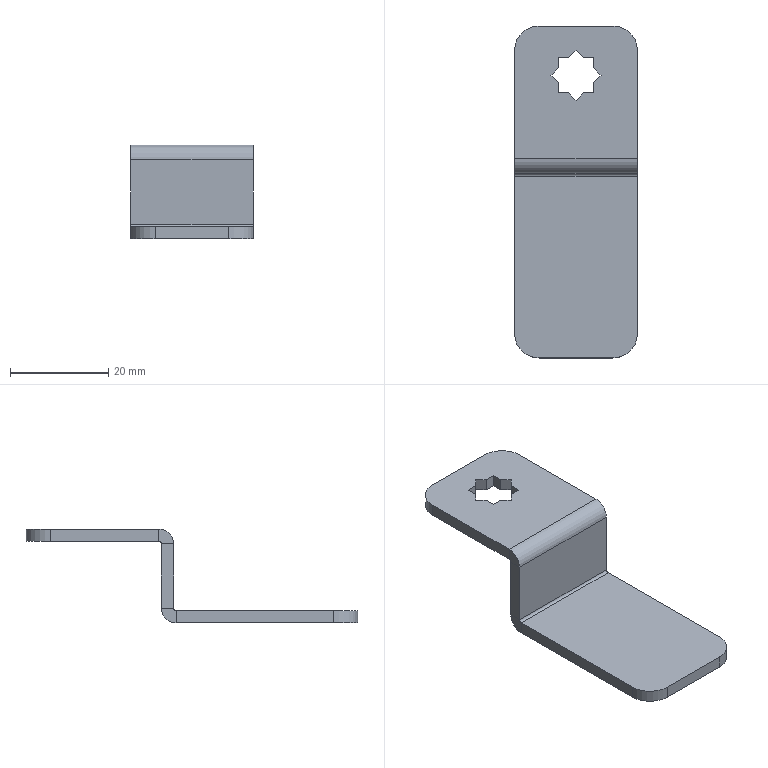Part | SolidWorks | features BaseBody 1 | 1 solid | 42 faces | box 25 x 67.5 x 19.1 mm | volume 4957 mm3 | plane 34 | cylinder 8 | commonest cylinder face diameters 10 x4 1 x2 6 x2
STEP:
#1=CARTESIAN_POINT('',(5.091,5.,0.));
#2=VERTEX_POINT('',#1);
#3=CARTESIAN_POINT('',(3.6,3.509,0.));
#4=VERTEX_POINT('',#3);
#5=CARTESIAN_POINT('',(5.091,5.,0.));
#6=DIRECTION('',(-0.7071,-0.7071,0.));
#7=VECTOR('',#6,1000.);
#8=LINE('',#5,#7);
#9=EDGE_CURVE('',#2,#4,#8,.T.);
#10=ORIENTED_EDGE('',*,*,#9,.F.);
#11=CARTESIAN_POINT('',(5.091,5.,-2.5));
#12=VERTEX_POINT('',#11);
#13=CARTESIAN_POINT('',(5.091,5.,0.));
#14=DIRECTION('',(0.,0.,-1.));
#15=VECTOR('',#14,1000.);
#16=LINE('',#13,#15);
#17=EDGE_CURVE('',#2,#12,#16,.T.);
#18=ORIENTED_EDGE('',*,*,#17,.T.);
#19=CARTESIAN_POINT('',(3.6,3.509,-2.5));
#20=VERTEX_POINT('',#19);
#21=CARTESIAN_POINT('',(5.091,5.,-2.5));
#22=DIRECTION('',(-0.7071,-0.7071,0.));
#23=VECTOR('',#22,1000.);
#24=LINE('',#21,#23);
#25=EDGE_CURVE('',#12,#20,#24,.T.);
#26=ORIENTED_EDGE('',*,*,#25,.T.);
#27=CARTESIAN_POINT('',(3.6,3.509,0.));
#28=DIRECTION('',(0.,0.,-1.));
#29=VECTOR('',#28,1000.);
#30=LINE('',#27,#29);
#31=EDGE_CURVE('',#4,#20,#30,.T.);
#32=ORIENTED_EDGE('',*,*,#31,.F.);
#33=EDGE_LOOP('',(#10,#18,#26,#32));
#34=FACE_OUTER_BOUND('',#33,.T.);
#35=CARTESIAN_POINT('',(5.091,5.,0.));
#36=DIRECTION('',(0.7071,-0.7071,0.));
#37=DIRECTION('',(0.,0.,-1.));
#38=AXIS2_PLACEMENT_3D('',#35,#36,#37);
#39=PLANE('',#38);
#40=ADVANCED_FACE('',(#34),#39,.F.);
#41=CARTESIAN_POINT('',(3.6,6.491,-2.5));
#42=VERTEX_POINT('',#41);
#43=CARTESIAN_POINT('',(0.,10.091,-2.5));
#44=DIRECTION('',(0.7071,-0.7071,0.));
#45=VECTOR('',#44,1000.);
#46=LINE('',#43,#45);
#47=EDGE_CURVE('',#42,#12,#46,.T.);
#48=ORIENTED_EDGE('',*,*,#47,.T.);
#49=ORIENTED_EDGE('',*,*,#17,.F.);
#50=CARTESIAN_POINT('',(3.6,6.491,0.));
#51=VERTEX_POINT('',#50);
#52=CARTESIAN_POINT('',(0.,10.091,0.));
#53=DIRECTION('',(0.7071,-0.7071,0.));
#54=VECTOR('',#53,1000.);
#55=LINE('',#52,#54);
#56=EDGE_CURVE('',#51,#2,#55,.T.);
#57=ORIENTED_EDGE('',*,*,#56,.F.);
#58=CARTESIAN_POINT('',(3.6,6.491,0.));
#59=DIRECTION('',(0.,0.,1.));
#60=VECTOR('',#59,1000.);
#61=LINE('',#58,#60);
#62=EDGE_CURVE('',#42,#51,#61,.T.);
#63=ORIENTED_EDGE('',*,*,#62,.F.);
#64=EDGE_LOOP('',(#48,#49,#57,#63));
#65=FACE_OUTER_BOUND('',#64,.T.);
#66=CARTESIAN_POINT('',(0.,10.091,0.));
#67=DIRECTION('',(0.7071,0.7071,0.));
#68=DIRECTION('',(0.,0.,-1.));
#69=AXIS2_PLACEMENT_3D('',#66,#67,#68);
#70=PLANE('',#69);
#71=ADVANCED_FACE('',(#65),#70,.F.);
#72=CARTESIAN_POINT('',(0.,10.091,0.));
#73=VERTEX_POINT('',#72);
#74=CARTESIAN_POINT('',(1.491,8.6,0.));
#75=VERTEX_POINT('',#74);
#76=CARTESIAN_POINT('',(0.,10.091,0.));
#77=DIRECTION('',(0.7071,-0.7071,0.));
#78=VECTOR('',#77,1000.);
#79=LINE('',#76,#78);
#80=EDGE_CURVE('',#73,#75,#79,.T.);
#81=ORIENTED_EDGE('',*,*,#80,.F.);
#82=CARTESIAN_POINT('',(0.,10.091,-2.5));
#83=VERTEX_POINT('',#82);
#84=CARTESIAN_POINT('',(0.,10.091,0.));
#85=DIRECTION('',(0.,0.,-1.));
#86=VECTOR('',#85,1000.);
#87=LINE('',#84,#86);
#88=EDGE_CURVE('',#73,#83,#87,.T.);
#89=ORIENTED_EDGE('',*,*,#88,.T.);
#90=CARTESIAN_POINT('',(1.491,8.6,-2.5));
#91=VERTEX_POINT('',#90);
#92=CARTESIAN_POINT('',(0.,10.091,-2.5));
#93=DIRECTION('',(0.7071,-0.7071,0.));
#94=VECTOR('',#93,1000.);
#95=LINE('',#92,#94);
#96=EDGE_CURVE('',#83,#91,#95,.T.);
#97=ORIENTED_EDGE('',*,*,#96,.T.);
#98=CARTESIAN_POINT('',(1.491,8.6,0.));
#99=DIRECTION('',(0.,0.,-1.));
#100=VECTOR('',#99,1000.);
#101=LINE('',#98,#100);
#102=EDGE_CURVE('',#75,#91,#101,.T.);
#103=ORIENTED_EDGE('',*,*,#102,.F.);
#104=EDGE_LOOP('',(#81,#89,#97,#103));
#105=FACE_OUTER_BOUND('',#104,.T.);
#106=CARTESIAN_POINT('',(0.,10.091,0.));
#107=DIRECTION('',(0.7071,0.7071,0.));
#108=DIRECTION('',(0.,0.,-1.));
#109=AXIS2_PLACEMENT_3D('',#106,#107,#108);
#110=PLANE('',#109);
#111=ADVANCED_FACE('',(#105),#110,.F.);
#112=CARTESIAN_POINT('',(-1.491,8.6,-2.5));
#113=VERTEX_POINT('',#112);
#114=CARTESIAN_POINT('',(0.,10.091,-2.5));
#115=DIRECTION('',(0.7071,0.7071,0.));
#116=VECTOR('',#115,1000.);
#117=LINE('',#114,#116);
#118=EDGE_CURVE('',#113,#83,#117,.T.);
#119=ORIENTED_EDGE('',*,*,#118,.T.);
#120=ORIENTED_EDGE('',*,*,#88,.F.);
#121=CARTESIAN_POINT('',(-1.491,8.6,0.));
#122=VERTEX_POINT('',#121);
#123=CARTESIAN_POINT('',(0.,10.091,0.));
#124=DIRECTION('',(0.7071,0.7071,0.));
#125=VECTOR('',#124,1000.);
#126=LINE('',#123,#125);
#127=EDGE_CURVE('',#122,#73,#126,.T.);
#128=ORIENTED_EDGE('',*,*,#127,.F.);
#129=CARTESIAN_POINT('',(-1.491,8.6,0.));
#130=DIRECTION('',(0.,0.,1.));
#131=VECTOR('',#130,1000.);
#132=LINE('',#129,#131);
#133=EDGE_CURVE('',#113,#122,#132,.T.);
#134=ORIENTED_EDGE('',*,*,#133,.F.);
#135=EDGE_LOOP('',(#119,#120,#128,#134));
#136=FACE_OUTER_BOUND('',#135,.T.);
#137=CARTESIAN_POINT('',(0.,10.091,0.));
#138=DIRECTION('',(-0.7071,0.7071,0.));
#139=DIRECTION('',(0.,0.,1.));
#140=AXIS2_PLACEMENT_3D('',#137,#138,#139);
#141=PLANE('',#140);
#142=ADVANCED_FACE('',(#136),#141,.F.);
#143=CARTESIAN_POINT('',(-5.091,5.,0.));
#144=VERTEX_POINT('',#143);
#145=CARTESIAN_POINT('',(-3.6,6.491,0.));
#146=VERTEX_POINT('',#145);
#147=CARTESIAN_POINT('',(0.,10.091,0.));
#148=DIRECTION('',(0.7071,0.7071,0.));
#149=VECTOR('',#148,1000.);
#150=LINE('',#147,#149);
#151=EDGE_CURVE('',#144,#146,#150,.T.);
#152=ORIENTED_EDGE('',*,*,#151,.F.);
#153=CARTESIAN_POINT('',(-5.091,5.,-2.5));
#154=VERTEX_POINT('',#153);
#155=CARTESIAN_POINT('',(-5.091,5.,0.));
#156=DIRECTION('',(0.,0.,-1.));
#157=VECTOR('',#156,1000.);
#158=LINE('',#155,#157);
#159=EDGE_CURVE('',#144,#154,#158,.T.);
#160=ORIENTED_EDGE('',*,*,#159,.T.);
#161=CARTESIAN_POINT('',(-3.6,6.491,-2.5));
#162=VERTEX_POINT('',#161);
#163=CARTESIAN_POINT('',(0.,10.091,-2.5));
#164=DIRECTION('',(0.7071,0.7071,0.));
#165=VECTOR('',#164,1000.);
#166=LINE('',#163,#165);
#167=EDGE_CURVE('',#154,#162,#166,.T.);
#168=ORIENTED_EDGE('',*,*,#167,.T.);
#169=CARTESIAN_POINT('',(-3.6,6.491,0.));
#170=DIRECTION('',(0.,0.,-1.));
#171=VECTOR('',#170,1000.);
#172=LINE('',#169,#171);
#173=EDGE_CURVE('',#146,#162,#172,.T.);
#174=ORIENTED_EDGE('',*,*,#173,.F.);
#175=EDGE_LOOP('',(#152,#160,#168,#174));
#176=FACE_OUTER_BOUND('',#175,.T.);
#177=CARTESIAN_POINT('',(0.,10.091,0.));
#178=DIRECTION('',(-0.7071,0.7071,0.));
#179=DIRECTION('',(0.,0.,1.));
#180=AXIS2_PLACEMENT_3D('',#177,#178,#179);
#181=PLANE('',#180);
#182=ADVANCED_FACE('',(#176),#181,.F.);
#183=CARTESIAN_POINT('',(-3.6,3.509,-2.5));
#184=VERTEX_POINT('',#183);
#185=CARTESIAN_POINT('',(-5.091,5.,-2.5));
#186=DIRECTION('',(-0.7071,0.7071,0.));
#187=VECTOR('',#186,1000.);
#188=LINE('',#185,#187);
#189=EDGE_CURVE('',#184,#154,#188,.T.);
#190=ORIENTED_EDGE('',*,*,#189,.T.);
#191=ORIENTED_EDGE('',*,*,#159,.F.);
#192=CARTESIAN_POINT('',(-3.6,3.509,0.));
#193=VERTEX_POINT('',#192);
#194=CARTESIAN_POINT('',(-5.091,5.,0.));
#195=DIRECTION('',(-0.7071,0.7071,0.));
#196=VECTOR('',#195,1000.);
#197=LINE('',#194,#196);
#198=EDGE_CURVE('',#193,#144,#197,.T.);
#199=ORIENTED_EDGE('',*,*,#198,.F.);
#200=CARTESIAN_POINT('',(-3.6,3.509,0.));
#201=DIRECTION('',(0.,0.,1.));
#202=VECTOR('',#201,1000.);
#203=LINE('',#200,#202);
#204=EDGE_CURVE('',#184,#193,#203,.T.);
#205=ORIENTED_EDGE('',*,*,#204,.F.);
#206=EDGE_LOOP('',(#190,#191,#199,#205));
#207=FACE_OUTER_BOUND('',#206,.T.);
#208=CARTESIAN_POINT('',(-5.091,5.,0.));
#209=DIRECTION('',(-0.7071,-0.7071,0.));
#210=DIRECTION('',(-0.7071,0.7071,0.));
#211=AXIS2_PLACEMENT_3D('',#208,#209,#210);
#212=PLANE('',#211);
#213=ADVANCED_FACE('',(#207),#212,.F.);
#214=CARTESIAN_POINT('',(1.491,1.4,-2.5));
#215=VERTEX_POINT('',#214);
#216=CARTESIAN_POINT('',(0.,-0.09117,-2.5));
#217=VERTEX_POINT('',#216);
#218=CARTESIAN_POINT('',(5.091,5.,-2.5));
#219=DIRECTION('',(-0.7071,-0.7071,0.));
#220=VECTOR('',#219,1000.);
#221=LINE('',#218,#220);
#222=EDGE_CURVE('',#215,#217,#221,.T.);
#223=ORIENTED_EDGE('',*,*,#222,.T.);
#224=CARTESIAN_POINT('',(0.,-0.09117,0.));
#225=VERTEX_POINT('',#224);
#226=CARTESIAN_POINT('',(0.,-0.09117,0.));
#227=DIRECTION('',(0.,0.,-1.));
#228=VECTOR('',#227,1000.);
#229=LINE('',#226,#228);
#230=EDGE_CURVE('',#225,#217,#229,.T.);
#231=ORIENTED_EDGE('',*,*,#230,.F.);
#232=CARTESIAN_POINT('',(1.491,1.4,0.));
#233=VERTEX_POINT('',#232);
#234=CARTESIAN_POINT('',(5.091,5.,0.));
#235=DIRECTION('',(-0.7071,-0.7071,0.));
#236=VECTOR('',#235,1000.);
#237=LINE('',#234,#236);
#238=EDGE_CURVE('',#233,#225,#237,.T.);
#239=ORIENTED_EDGE('',*,*,#238,.F.);
#240=CARTESIAN_POINT('',(1.491,1.4,0.));
#241=DIRECTION('',(0.,0.,1.));
#242=VECTOR('',#241,1000.);
#243=LINE('',#240,#242);
#244=EDGE_CURVE('',#215,#233,#243,.T.);
#245=ORIENTED_EDGE('',*,*,#244,.F.);
#246=EDGE_LOOP('',(#223,#231,#239,#245));
#247=FACE_OUTER_BOUND('',#246,.T.);
#248=CARTESIAN_POINT('',(5.091,5.,0.));
#249=DIRECTION('',(0.7071,-0.7071,0.));
#250=DIRECTION('',(0.,0.,-1.));
#251=AXIS2_PLACEMENT_3D('',#248,#249,#250);
#252=PLANE('',#251);
#253=ADVANCED_FACE('',(#247),#252,.F.);
#254=CARTESIAN_POINT('',(-1.491,1.4,0.));
#255=VERTEX_POINT('',#254);
#256=CARTESIAN_POINT('',(-5.091,5.,0.));
#257=DIRECTION('',(-0.7071,0.7071,0.));
#258=VECTOR('',#257,1000.);
#259=LINE('',#256,#258);
#260=EDGE_CURVE('',#225,#255,#259,.T.);
#261=ORIENTED_EDGE('',*,*,#260,.F.);
#262=ORIENTED_EDGE('',*,*,#230,.T.);
#263=CARTESIAN_POINT('',(-1.491,1.4,-2.5));
#264=VERTEX_POINT('',#263);
#265=CARTESIAN_POINT('',(-5.091,5.,-2.5));
#266=DIRECTION('',(-0.7071,0.7071,0.));
#267=VECTOR('',#266,1000.);
#268=LINE('',#265,#267);
#269=EDGE_CURVE('',#217,#264,#268,.T.);
#270=ORIENTED_EDGE('',*,*,#269,.T.);
#271=CARTESIAN_POINT('',(-1.491,1.4,0.));
#272=DIRECTION('',(0.,0.,-1.));
#273=VECTOR('',#272,1000.);
#274=LINE('',#271,#273);
#275=EDGE_CURVE('',#255,#264,#274,.T.);
#276=ORIENTED_EDGE('',*,*,#275,.F.);
#277=EDGE_LOOP('',(#261,#262,#270,#276));
#278=FACE_OUTER_BOUND('',#277,.T.);
#279=CARTESIAN_POINT('',(-5.091,5.,0.));
#280=DIRECTION('',(-0.7071,-0.7071,0.));
#281=DIRECTION('',(-0.7071,0.7071,0.));
#282=AXIS2_PLACEMENT_3D('',#279,#280,#281);
#283=PLANE('',#282);
#284=ADVANCED_FACE('',(#278),#283,.F.);
#285=CARTESIAN_POINT('',(-3.6,1.4,0.));
#286=VERTEX_POINT('',#285);
#287=CARTESIAN_POINT('',(-3.6,1.4,0.));
#288=DIRECTION('',(-1.,0.,0.));
#289=VECTOR('',#288,1000.);
#290=LINE('',#287,#289);
#291=EDGE_CURVE('',#255,#286,#290,.T.);
#292=ORIENTED_EDGE('',*,*,#291,.F.);
#293=ORIENTED_EDGE('',*,*,#275,.T.);
#294=CARTESIAN_POINT('',(-3.6,1.4,-2.5));
#295=VERTEX_POINT('',#294);
#296=CARTESIAN_POINT('',(-3.6,1.4,-2.5));
#297=DIRECTION('',(-1.,0.,0.));
#298=VECTOR('',#297,1000.);
#299=LINE('',#296,#298);
#300=EDGE_CURVE('',#264,#295,#299,.T.);
#301=ORIENTED_EDGE('',*,*,#300,.T.);
#302=CARTESIAN_POINT('',(-3.6,1.4,0.));
#303=DIRECTION('',(0.,0.,-1.));
#304=VECTOR('',#303,1000.);
#305=LINE('',#302,#304);
#306=EDGE_CURVE('',#286,#295,#305,.T.);
#307=ORIENTED_EDGE('',*,*,#306,.F.);
#308=EDGE_LOOP('',(#292,#293,#301,#307));
#309=FACE_OUTER_BOUND('',#308,.T.);
#310=CARTESIAN_POINT('',(-3.6,1.4,0.));
#311=DIRECTION('',(0.,-1.,0.));
#312=DIRECTION('',(-1.,0.,0.));
#313=AXIS2_PLACEMENT_3D('',#310,#311,#312);
#314=PLANE('',#313);
#315=ADVANCED_FACE('',(#309),#314,.F.);
#316=CARTESIAN_POINT('',(-3.6,8.6,-2.5));
#317=DIRECTION('',(0.,1.,0.));
#318=VECTOR('',#317,1000.);
#319=LINE('',#316,#318);
#320=EDGE_CURVE('',#295,#184,#319,.T.);
#321=ORIENTED_EDGE('',*,*,#320,.T.);
#322=ORIENTED_EDGE('',*,*,#204,.T.);
#323=CARTESIAN_POINT('',(-3.6,8.6,0.));
#324=DIRECTION('',(0.,1.,0.));
#325=VECTOR('',#324,1000.);
#326=LINE('',#323,#325);
#327=EDGE_CURVE('',#286,#193,#326,.T.);
#328=ORIENTED_EDGE('',*,*,#327,.F.);
#329=ORIENTED_EDGE('',*,*,#306,.T.);
#330=EDGE_LOOP('',(#321,#322,#328,#329));
#331=FACE_OUTER_BOUND('',#330,.T.);
#332=CARTESIAN_POINT('',(-3.6,8.6,0.));
#333=DIRECTION('',(-1.,0.,0.));
#334=DIRECTION('',(0.,0.,1.));
#335=AXIS2_PLACEMENT_3D('',#332,#333,#334);
#336=PLANE('',#335);
#337=ADVANCED_FACE('',(#331),#336,.F.);
#338=CARTESIAN_POINT('',(-3.6,8.6,-2.5));
#339=VERTEX_POINT('',#338);
#340=CARTESIAN_POINT('',(-3.6,8.6,-2.5));
#341=DIRECTION('',(1.,0.,0.));
#342=VECTOR('',#341,1000.);
#343=LINE('',#340,#342);
#344=EDGE_CURVE('',#339,#113,#343,.T.);
#345=ORIENTED_EDGE('',*,*,#344,.T.);
#346=ORIENTED_EDGE('',*,*,#133,.T.);
#347=CARTESIAN_POINT('',(-3.6,8.6,0.));
#348=VERTEX_POINT('',#347);
#349=CARTESIAN_POINT('',(-3.6,8.6,0.));
#350=DIRECTION('',(1.,0.,0.));
#351=VECTOR('',#350,1000.);
#352=LINE('',#349,#351);
#353=EDGE_CURVE('',#348,#122,#352,.T.);
#354=ORIENTED_EDGE('',*,*,#353,.F.);
#355=CARTESIAN_POINT('',(-3.6,8.6,0.));
#356=DIRECTION('',(0.,0.,-1.));
#357=VECTOR('',#356,1000.);
#358=LINE('',#355,#357);
#359=EDGE_CURVE('',#348,#339,#358,.T.);
#360=ORIENTED_EDGE('',*,*,#359,.T.);
#361=EDGE_LOOP('',(#345,#346,#354,#360));
#362=FACE_OUTER_BOUND('',#361,.T.);
#363=CARTESIAN_POINT('',(-3.6,8.6,0.));
#364=DIRECTION('',(0.,1.,0.));
#365=DIRECTION('',(0.,0.,-1.));
#366=AXIS2_PLACEMENT_3D('',#363,#364,#365);
#367=PLANE('',#366);
#368=ADVANCED_FACE('',(#362),#367,.F.);
#369=CARTESIAN_POINT('',(3.6,8.6,-2.5));
#370=VERTEX_POINT('',#369);
#371=CARTESIAN_POINT('',(3.6,8.6,-2.5));
#372=DIRECTION('',(0.,-1.,0.));
#373=VECTOR('',#372,1000.);
#374=LINE('',#371,#373);
#375=EDGE_CURVE('',#370,#42,#374,.T.);
#376=ORIENTED_EDGE('',*,*,#375,.T.);
#377=ORIENTED_EDGE('',*,*,#62,.T.);
#378=CARTESIAN_POINT('',(3.6,8.6,0.));
#379=VERTEX_POINT('',#378);
#380=CARTESIAN_POINT('',(3.6,8.6,0.));
#381=DIRECTION('',(0.,-1.,0.));
#382=VECTOR('',#381,1000.);
#383=LINE('',#380,#382);
#384=EDGE_CURVE('',#379,#51,#383,.T.);
#385=ORIENTED_EDGE('',*,*,#384,.F.);
#386=CARTESIAN_POINT('',(3.6,8.6,0.));
#387=DIRECTION('',(0.,0.,-1.));
#388=VECTOR('',#387,1000.);
#389=LINE('',#386,#388);
#390=EDGE_CURVE('',#379,#370,#389,.T.);
#391=ORIENTED_EDGE('',*,*,#390,.T.);
#392=EDGE_LOOP('',(#376,#377,#385,#391));
#393=FACE_OUTER_BOUND('',#392,.T.);
#394=CARTESIAN_POINT('',(3.6,8.6,0.));
#395=DIRECTION('',(1.,0.,0.));
#396=DIRECTION('',(0.,1.,0.));
#397=AXIS2_PLACEMENT_3D('',#394,#395,#396);
#398=PLANE('',#397);
#399=ADVANCED_FACE('',(#393),#398,.F.);
#400=CARTESIAN_POINT('',(-7.5,-52.5,-19.1));
#401=VERTEX_POINT('',#400);
#402=CARTESIAN_POINT('',(-12.5,-47.5,-19.1));
#403=VERTEX_POINT('',#402);
#404=CARTESIAN_POINT('',(-7.5,-47.5,-19.1));
#405=DIRECTION('',(0.,0.,-1.));
#406=DIRECTION('',(1.,0.,0.));
#407=AXIS2_PLACEMENT_3D('',#404,#405,#406);
#408=CIRCLE('',#407,5.);
#409=EDGE_CURVE('',#401,#403,#408,.T.);
#410=ORIENTED_EDGE('',*,*,#409,.F.);
#411=CARTESIAN_POINT('',(-7.5,-52.5,-16.6));
#412=VERTEX_POINT('',#411);
#413=CARTESIAN_POINT('',(-7.5,-52.5,-19.1));
#414=DIRECTION('',(0.,0.,-1.));
#415=VECTOR('',#414,1000.);
#416=LINE('',#413,#415);
#417=EDGE_CURVE('',#412,#401,#416,.T.);
#418=ORIENTED_EDGE('',*,*,#417,.F.);
#419=CARTESIAN_POINT('',(-12.5,-47.5,-16.6));
#420=VERTEX_POINT('',#419);
#421=CARTESIAN_POINT('',(-7.5,-47.5,-16.6));
#422=DIRECTION('',(0.,0.,1.));
#423=DIRECTION('',(1.,0.,0.));
#424=AXIS2_PLACEMENT_3D('',#421,#422,#423);
#425=CIRCLE('',#424,5.);
#426=EDGE_CURVE('',#420,#412,#425,.T.);
#427=ORIENTED_EDGE('',*,*,#426,.F.);
#428=CARTESIAN_POINT('',(-12.5,-47.5,-19.1));
#429=DIRECTION('',(0.,0.,1.));
#430=VECTOR('',#429,1000.);
#431=LINE('',#428,#430);
#432=EDGE_CURVE('',#403,#420,#431,.T.);
#433=ORIENTED_EDGE('',*,*,#432,.F.);
#434=EDGE_LOOP('',(#410,#418,#427,#433));
#435=FACE_OUTER_BOUND('',#434,.T.);
#436=CARTESIAN_POINT('',(-7.5,-47.5,-19.1));
#437=DIRECTION('',(0.,0.,1.));
#438=DIRECTION('',(0.,-1.,0.));
#439=AXIS2_PLACEMENT_3D('',#436,#437,#438);
#440=CYLINDRICAL_SURFACE('',#439,5.);
#441=ADVANCED_FACE('',(#435),#440,.T.);
#442=CARTESIAN_POINT('',(-12.5,10.,-2.5));
#443=VERTEX_POINT('',#442);
#444=CARTESIAN_POINT('',(-7.5,15.,-2.5));
#445=VERTEX_POINT('',#444);
#446=CARTESIAN_POINT('',(-7.5,10.,-2.5));
#447=DIRECTION('',(0.,0.,-1.));
#448=DIRECTION('',(-1.,0.,0.));
#449=AXIS2_PLACEMENT_3D('',#446,#447,#448);
#450=CIRCLE('',#449,5.);
#451=EDGE_CURVE('',#443,#445,#450,.T.);
#452=ORIENTED_EDGE('',*,*,#451,.F.);
#453=CARTESIAN_POINT('',(-12.5,10.,0.));
#454=VERTEX_POINT('',#453);
#455=CARTESIAN_POINT('',(-12.5,10.,-2.5));
#456=DIRECTION('',(0.,0.,-1.));
#457=VECTOR('',#456,1000.);
#458=LINE('',#455,#457);
#459=EDGE_CURVE('',#454,#443,#458,.T.);
#460=ORIENTED_EDGE('',*,*,#459,.F.);
#461=CARTESIAN_POINT('',(-7.5,15.,0.));
#462=VERTEX_POINT('',#461);
#463=CARTESIAN_POINT('',(-7.5,10.,0.));
#464=DIRECTION('',(0.,0.,1.));
#465=DIRECTION('',(-1.,0.,0.));
#466=AXIS2_PLACEMENT_3D('',#463,#464,#465);
#467=CIRCLE('',#466,5.);
#468=EDGE_CURVE('',#462,#454,#467,.T.);
#469=ORIENTED_EDGE('',*,*,#468,.F.);
#470=CARTESIAN_POINT('',(-7.5,15.,-2.5));
#471=DIRECTION('',(0.,0.,1.));
#472=VECTOR('',#471,1000.);
#473=LINE('',#470,#472);
#474=EDGE_CURVE('',#445,#462,#473,.T.);
#475=ORIENTED_EDGE('',*,*,#474,.F.);
#476=EDGE_LOOP('',(#452,#460,#469,#475));
#477=FACE_OUTER_BOUND('',#476,.T.);
#478=CARTESIAN_POINT('',(-7.5,10.,-2.5));
#479=DIRECTION('',(0.,0.,1.));
#480=DIRECTION('',(1.,0.,0.));
#481=AXIS2_PLACEMENT_3D('',#478,#479,#480);
#482=CYLINDRICAL_SURFACE('',#481,5.);
#483=ADVANCED_FACE('',(#477),#482,.T.);
#484=CARTESIAN_POINT('',(7.5,15.,-2.5));
#485=VERTEX_POINT('',#484);
#486=CARTESIAN_POINT('',(12.5,10.,-2.5));
#487=VERTEX_POINT('',#486);
#488=CARTESIAN_POINT('',(7.5,10.,-2.5));
#489=DIRECTION('',(0.,0.,-1.));
#490=DIRECTION('',(-1.,0.,0.));
#491=AXIS2_PLACEMENT_3D('',#488,#489,#490);
#492=CIRCLE('',#491,5.);
#493=EDGE_CURVE('',#485,#487,#492,.T.);
#494=ORIENTED_EDGE('',*,*,#493,.F.);
#495=CARTESIAN_POINT('',(7.5,15.,0.));
#496=VERTEX_POINT('',#495);
#497=CARTESIAN_POINT('',(7.5,15.,-2.5));
#498=DIRECTION('',(0.,0.,-1.));
#499=VECTOR('',#498,1000.);
#500=LINE('',#497,#499);
#501=EDGE_CURVE('',#496,#485,#500,.T.);
#502=ORIENTED_EDGE('',*,*,#501,.F.);
#503=CARTESIAN_POINT('',(12.5,10.,0.));
#504=VERTEX_POINT('',#503);
#505=CARTESIAN_POINT('',(7.5,10.,0.));
#506=DIRECTION('',(0.,0.,1.));
#507=DIRECTION('',(-1.,0.,0.));
#508=AXIS2_PLACEMENT_3D('',#505,#506,#507);
#509=CIRCLE('',#508,5.);
#510=EDGE_CURVE('',#504,#496,#509,.T.);
#511=ORIENTED_EDGE('',*,*,#510,.F.);
#512=CARTESIAN_POINT('',(12.5,10.,-2.5));
#513=DIRECTION('',(0.,0.,1.));
#514=VECTOR('',#513,1000.);
#515=LINE('',#512,#514);
#516=EDGE_CURVE('',#487,#504,#515,.T.);
#517=ORIENTED_EDGE('',*,*,#516,.F.);
#518=EDGE_LOOP('',(#494,#502,#511,#517));
#519=FACE_OUTER_BOUND('',#518,.T.);
#520=CARTESIAN_POINT('',(7.5,10.,-2.5));
#521=DIRECTION('',(0.,0.,1.));
#522=DIRECTION('',(1.,0.,0.));
#523=AXIS2_PLACEMENT_3D('',#520,#521,#522);
#524=CYLINDRICAL_SURFACE('',#523,5.);
#525=ADVANCED_FACE('',(#519),#524,.T.);
#526=CARTESIAN_POINT('',(12.5,-47.5,-19.1));
#527=VERTEX_POINT('',#526);
#528=CARTESIAN_POINT('',(7.5,-52.5,-19.1));
#529=VERTEX_POINT('',#528);
#530=CARTESIAN_POINT('',(7.5,-47.5,-19.1));
#531=DIRECTION('',(0.,0.,-1.));
#532=DIRECTION('',(1.,0.,0.));
#533=AXIS2_PLACEMENT_3D('',#530,#531,#532);
#534=CIRCLE('',#533,5.);
#535=EDGE_CURVE('',#527,#529,#534,.T.);
#536=ORIENTED_EDGE('',*,*,#535,.F.);
#537=CARTESIAN_POINT('',(12.5,-47.5,-16.6));
#538=VERTEX_POINT('',#537);
#539=CARTESIAN_POINT('',(12.5,-47.5,-19.1));
#540=DIRECTION('',(0.,0.,-1.));
#541=VECTOR('',#540,1000.);
#542=LINE('',#539,#541);
#543=EDGE_CURVE('',#538,#527,#542,.T.);
#544=ORIENTED_EDGE('',*,*,#543,.F.);
#545=CARTESIAN_POINT('',(7.5,-52.5,-16.6));
#546=VERTEX_POINT('',#545);
#547=CARTESIAN_POINT('',(7.5,-47.5,-16.6));
#548=DIRECTION('',(0.,0.,1.));
#549=DIRECTION('',(1.,0.,0.));
#550=AXIS2_PLACEMENT_3D('',#547,#548,#549);
#551=CIRCLE('',#550,5.);
#552=EDGE_CURVE('',#546,#538,#551,.T.);
#553=ORIENTED_EDGE('',*,*,#552,.F.);
#554=CARTESIAN_POINT('',(7.5,-52.5,-19.1));
#555=DIRECTION('',(0.,0.,1.));
#556=VECTOR('',#555,1000.);
#557=LINE('',#554,#556);
#558=EDGE_CURVE('',#529,#546,#557,.T.);
#559=ORIENTED_EDGE('',*,*,#558,.F.);
#560=EDGE_LOOP('',(#536,#544,#553,#559));
#561=FACE_OUTER_BOUND('',#560,.T.);
#562=CARTESIAN_POINT('',(7.5,-47.5,-19.1));
#563=DIRECTION('',(0.,0.,1.));
#564=DIRECTION('',(0.,-1.,0.));
#565=AXIS2_PLACEMENT_3D('',#562,#563,#564);
#566=CYLINDRICAL_SURFACE('',#565,5.);
#567=ADVANCED_FACE('',(#561),#566,.T.);
#568=CARTESIAN_POINT('',(0.,-52.5,-19.1));
#569=DIRECTION('',(-1.,0.,0.));
#570=VECTOR('',#569,1000.);
#571=LINE('',#568,#570);
#572=EDGE_CURVE('',#529,#401,#571,.T.);
#573=ORIENTED_EDGE('',*,*,#572,.F.);
#574=ORIENTED_EDGE('',*,*,#558,.T.);
#575=CARTESIAN_POINT('',(-12.5,-52.5,-16.6));
#576=DIRECTION('',(-1.,0.,0.));
#577=VECTOR('',#576,1000.);
#578=LINE('',#575,#577);
#579=EDGE_CURVE('',#546,#412,#578,.T.);
#580=ORIENTED_EDGE('',*,*,#579,.T.);
#581=ORIENTED_EDGE('',*,*,#417,.T.);
#582=EDGE_LOOP('',(#573,#574,#580,#581));
#583=FACE_OUTER_BOUND('',#582,.T.);
#584=CARTESIAN_POINT('',(-12.5,-52.5,-19.1));
#585=DIRECTION('',(0.,1.,0.));
#586=DIRECTION('',(0.,0.,-1.));
#587=AXIS2_PLACEMENT_3D('',#584,#585,#586);
#588=PLANE('',#587);
#589=ADVANCED_FACE('',(#583),#588,.F.);
#590=ORIENTED_EDGE('',*,*,#579,.F.);
#591=ORIENTED_EDGE('',*,*,#552,.T.);
#592=CARTESIAN_POINT('',(12.5,-15.5,-16.6));
#593=VERTEX_POINT('',#592);
#594=CARTESIAN_POINT('',(12.5,-52.5,-16.6));
#595=DIRECTION('',(0.,-1.,0.));
#596=VECTOR('',#595,1000.);
#597=LINE('',#594,#596);
#598=EDGE_CURVE('',#593,#538,#597,.T.);
#599=ORIENTED_EDGE('',*,*,#598,.F.);
#600=CARTESIAN_POINT('',(-12.5,-15.5,-16.6));
#601=VERTEX_POINT('',#600);
#602=CARTESIAN_POINT('',(-12.5,-15.5,-16.6));
#603=DIRECTION('',(1.,0.,0.));
#604=VECTOR('',#603,1000.);
#605=LINE('',#602,#604);
#606=EDGE_CURVE('',#601,#593,#605,.T.);
#607=ORIENTED_EDGE('',*,*,#606,.F.);
#608=CARTESIAN_POINT('',(-12.5,-15.,-16.6));
#609=DIRECTION('',(0.,1.,0.));
#610=VECTOR('',#609,1000.);
#611=LINE('',#608,#610);
#612=EDGE_CURVE('',#420,#601,#611,.T.);
#613=ORIENTED_EDGE('',*,*,#612,.F.);
#614=ORIENTED_EDGE('',*,*,#426,.T.);
#615=EDGE_LOOP('',(#590,#591,#599,#607,#613,#614));
#616=FACE_OUTER_BOUND('',#615,.T.);
#617=CARTESIAN_POINT('',(0.,0.,-16.6));
#618=DIRECTION('',(0.,0.,1.));
#619=DIRECTION('',(1.,0.,0.));
#620=AXIS2_PLACEMENT_3D('',#617,#618,#619);
#621=PLANE('',#620);
#622=ADVANCED_FACE('',(#616),#621,.T.);
#623=CARTESIAN_POINT('',(12.5,-15.5,-19.1));
#624=VERTEX_POINT('',#623);
#625=CARTESIAN_POINT('',(12.5,0.,-19.1));
#626=DIRECTION('',(0.,-1.,0.));
#627=VECTOR('',#626,1000.);
#628=LINE('',#625,#627);
#629=EDGE_CURVE('',#624,#527,#628,.T.);
#630=ORIENTED_EDGE('',*,*,#629,.T.);
#631=ORIENTED_EDGE('',*,*,#535,.T.);
#632=ORIENTED_EDGE('',*,*,#572,.T.);
#633=ORIENTED_EDGE('',*,*,#409,.T.);
#634=CARTESIAN_POINT('',(-12.5,-15.5,-19.1));
#635=VERTEX_POINT('',#634);
#636=CARTESIAN_POINT('',(-12.5,0.,-19.1));
#637=DIRECTION('',(0.,1.,0.));
#638=VECTOR('',#637,1000.);
#639=LINE('',#636,#638);
#640=EDGE_CURVE('',#403,#635,#639,.T.);
#641=ORIENTED_EDGE('',*,*,#640,.T.);
#642=CARTESIAN_POINT('',(-12.5,-15.5,-19.1));
#643=DIRECTION('',(-1.,0.,0.));
#644=VECTOR('',#643,1000.);
#645=LINE('',#642,#644);
#646=EDGE_CURVE('',#624,#635,#645,.T.);
#647=ORIENTED_EDGE('',*,*,#646,.F.);
#648=EDGE_LOOP('',(#630,#631,#632,#633,#641,#647));
#649=FACE_OUTER_BOUND('',#648,.T.);
#650=CARTESIAN_POINT('',(0.,0.,-19.1));
#651=DIRECTION('',(0.,0.,1.));
#652=DIRECTION('',(1.,0.,0.));
#653=AXIS2_PLACEMENT_3D('',#650,#651,#652);
#654=PLANE('',#653);
#655=ADVANCED_FACE('',(#649),#654,.F.);
#656=ORIENTED_EDGE('',*,*,#640,.F.);
#657=ORIENTED_EDGE('',*,*,#432,.T.);
#658=ORIENTED_EDGE('',*,*,#612,.T.);
#659=CARTESIAN_POINT('',(-12.5,-15.5,-19.1));
#660=DIRECTION('',(0.,0.,-1.));
#661=VECTOR('',#660,1000.);
#662=LINE('',#659,#661);
#663=EDGE_CURVE('',#601,#635,#662,.T.);
#664=ORIENTED_EDGE('',*,*,#663,.T.);
#665=EDGE_LOOP('',(#656,#657,#658,#664));
#666=FACE_OUTER_BOUND('',#665,.T.);
#667=CARTESIAN_POINT('',(-12.5,-15.,-19.1));
#668=DIRECTION('',(1.,0.,0.));
#669=DIRECTION('',(0.,1.,0.));
#670=AXIS2_PLACEMENT_3D('',#667,#668,#669);
#671=PLANE('',#670);
#672=ADVANCED_FACE('',(#666),#671,.F.);
#673=ORIENTED_EDGE('',*,*,#598,.T.);
#674=ORIENTED_EDGE('',*,*,#543,.T.);
#675=ORIENTED_EDGE('',*,*,#629,.F.);
#676=CARTESIAN_POINT('',(12.5,-15.5,-16.6));
#677=DIRECTION('',(0.,0.,-1.));
#678=VECTOR('',#677,1000.);
#679=LINE('',#676,#678);
#680=EDGE_CURVE('',#593,#624,#679,.T.);
#681=ORIENTED_EDGE('',*,*,#680,.F.);
#682=EDGE_LOOP('',(#673,#674,#675,#681));
#683=FACE_OUTER_BOUND('',#682,.T.);
#684=CARTESIAN_POINT('',(12.5,-52.5,-19.1));
#685=DIRECTION('',(-1.,0.,0.));
#686=DIRECTION('',(0.,0.,1.));
#687=AXIS2_PLACEMENT_3D('',#684,#685,#686);
#688=PLANE('',#687);
#689=ADVANCED_FACE('',(#683),#688,.F.);
#690=CARTESIAN_POINT('',(12.5,-15.,-16.1));
#691=VERTEX_POINT('',#690);
#692=CARTESIAN_POINT('',(-12.5,-15.,-16.1));
#693=VERTEX_POINT('',#692);
#694=CARTESIAN_POINT('',(12.5,-15.,-16.1));
#695=DIRECTION('',(-1.,0.,0.));
#696=VECTOR('',#695,1000.);
#697=LINE('',#694,#696);
#698=EDGE_CURVE('',#691,#693,#697,.T.);
#699=ORIENTED_EDGE('',*,*,#698,.T.);
#700=CARTESIAN_POINT('',(-12.5,-15.5,-16.1));
#701=DIRECTION('',(-1.,0.,0.));
#702=DIRECTION('',(0.,0.,-1.));
#703=AXIS2_PLACEMENT_3D('',#700,#701,#702);
#704=CIRCLE('',#703,0.5);
#705=EDGE_CURVE('',#693,#601,#704,.T.);
#706=ORIENTED_EDGE('',*,*,#705,.T.);
#707=ORIENTED_EDGE('',*,*,#606,.T.);
#708=CARTESIAN_POINT('',(12.5,-15.5,-16.1));
#709=DIRECTION('',(1.,0.,0.));
#710=DIRECTION('',(0.,0.,-1.));
#711=AXIS2_PLACEMENT_3D('',#708,#709,#710);
#712=CIRCLE('',#711,0.5);
#713=EDGE_CURVE('',#593,#691,#712,.T.);
#714=ORIENTED_EDGE('',*,*,#713,.T.);
#715=EDGE_LOOP('',(#699,#706,#707,#714));
#716=FACE_OUTER_BOUND('',#715,.T.);
#717=CARTESIAN_POINT('',(12.5,-15.5,-16.1));
#718=DIRECTION('',(1.,0.,0.));
#719=DIRECTION('',(0.,0.,-1.));
#720=AXIS2_PLACEMENT_3D('',#717,#718,#719);
#721=CYLINDRICAL_SURFACE('',#720,0.5);
#722=ADVANCED_FACE('',(#716),#721,.F.);
#723=CARTESIAN_POINT('',(12.5,-12.5,-16.1));
#724=VERTEX_POINT('',#723);
#725=CARTESIAN_POINT('',(-12.5,-12.5,-16.1));
#726=VERTEX_POINT('',#725);
#727=CARTESIAN_POINT('',(12.5,-12.5,-16.1));
#728=DIRECTION('',(-1.,0.,0.));
#729=VECTOR('',#728,1000.);
#730=LINE('',#727,#729);
#731=EDGE_CURVE('',#724,#726,#730,.T.);
#732=ORIENTED_EDGE('',*,*,#731,.F.);
#733=CARTESIAN_POINT('',(12.5,-15.5,-16.1));
#734=DIRECTION('',(1.,0.,0.));
#735=DIRECTION('',(0.,0.,-1.));
#736=AXIS2_PLACEMENT_3D('',#733,#734,#735);
#737=CIRCLE('',#736,3.);
#738=EDGE_CURVE('',#624,#724,#737,.T.);
#739=ORIENTED_EDGE('',*,*,#738,.F.);
#740=ORIENTED_EDGE('',*,*,#646,.T.);
#741=CARTESIAN_POINT('',(-12.5,-15.5,-16.1));
#742=DIRECTION('',(-1.,0.,0.));
#743=DIRECTION('',(0.,0.,-1.));
#744=AXIS2_PLACEMENT_3D('',#741,#742,#743);
#745=CIRCLE('',#744,3.);
#746=EDGE_CURVE('',#726,#635,#745,.T.);
#747=ORIENTED_EDGE('',*,*,#746,.F.);
#748=EDGE_LOOP('',(#732,#739,#740,#747));
#749=FACE_OUTER_BOUND('',#748,.T.);
#750=CARTESIAN_POINT('',(12.5,-15.5,-16.1));
#751=DIRECTION('',(1.,0.,0.));
#752=DIRECTION('',(0.,0.,-1.));
#753=AXIS2_PLACEMENT_3D('',#750,#751,#752);
#754=CYLINDRICAL_SURFACE('',#753,3.);
#755=ADVANCED_FACE('',(#749),#754,.T.);
#756=ORIENTED_EDGE('',*,*,#713,.F.);
#757=ORIENTED_EDGE('',*,*,#680,.T.);
#758=ORIENTED_EDGE('',*,*,#738,.T.);
#759=CARTESIAN_POINT('',(12.5,-15.,-16.1));
#760=DIRECTION('',(0.,1.,0.));
#761=VECTOR('',#760,1000.);
#762=LINE('',#759,#761);
#763=EDGE_CURVE('',#691,#724,#762,.T.);
#764=ORIENTED_EDGE('',*,*,#763,.F.);
#765=EDGE_LOOP('',(#756,#757,#758,#764));
#766=FACE_OUTER_BOUND('',#765,.T.);
#767=CARTESIAN_POINT('',(12.5,-15.5,-16.1));
#768=DIRECTION('',(-1.,0.,0.));
#769=DIRECTION('',(0.,0.,1.));
#770=AXIS2_PLACEMENT_3D('',#767,#768,#769);
#771=PLANE('',#770);
#772=ADVANCED_FACE('',(#766),#771,.F.);
#773=ORIENTED_EDGE('',*,*,#663,.F.);
#774=ORIENTED_EDGE('',*,*,#705,.F.);
#775=CARTESIAN_POINT('',(-12.5,-15.,-16.1));
#776=DIRECTION('',(0.,1.,0.));
#777=VECTOR('',#776,1000.);
#778=LINE('',#775,#777);
#779=EDGE_CURVE('',#693,#726,#778,.T.);
#780=ORIENTED_EDGE('',*,*,#779,.T.);
#781=ORIENTED_EDGE('',*,*,#746,.T.);
#782=EDGE_LOOP('',(#773,#774,#780,#781));
#783=FACE_OUTER_BOUND('',#782,.T.);
#784=CARTESIAN_POINT('',(-12.5,-15.5,-16.1));
#785=DIRECTION('',(-1.,0.,0.));
#786=DIRECTION('',(0.,0.,1.));
#787=AXIS2_PLACEMENT_3D('',#784,#785,#786);
#788=PLANE('',#787);
#789=ADVANCED_FACE('',(#783),#788,.T.);
#790=CARTESIAN_POINT('',(-12.5,-12.,-2.5));
#791=VERTEX_POINT('',#790);
#792=CARTESIAN_POINT('',(12.5,-12.,-2.5));
#793=VERTEX_POINT('',#792);
#794=CARTESIAN_POINT('',(-12.5,-12.,-2.5));
#795=DIRECTION('',(1.,0.,0.));
#796=VECTOR('',#795,1000.);
#797=LINE('',#794,#796);
#798=EDGE_CURVE('',#791,#793,#797,.T.);
#799=ORIENTED_EDGE('',*,*,#798,.T.);
#800=CARTESIAN_POINT('',(12.5,-12.5,-3.));
#801=VERTEX_POINT('',#800);
#802=CARTESIAN_POINT('',(12.5,-12.,-3.));
#803=DIRECTION('',(1.,0.,0.));
#804=DIRECTION('',(0.,0.,1.));
#805=AXIS2_PLACEMENT_3D('',#802,#803,#804);
#806=CIRCLE('',#805,0.5);
#807=EDGE_CURVE('',#793,#801,#806,.T.);
#808=ORIENTED_EDGE('',*,*,#807,.T.);
#809=CARTESIAN_POINT('',(-12.5,-12.5,-3.));
#810=VERTEX_POINT('',#809);
#811=CARTESIAN_POINT('',(12.5,-12.5,-3.));
#812=DIRECTION('',(-1.,0.,0.));
#813=VECTOR('',#812,1000.);
#814=LINE('',#811,#813);
#815=EDGE_CURVE('',#801,#810,#814,.T.);
#816=ORIENTED_EDGE('',*,*,#815,.T.);
#817=CARTESIAN_POINT('',(-12.5,-12.,-3.));
#818=DIRECTION('',(-1.,0.,0.));
#819=DIRECTION('',(0.,0.,1.));
#820=AXIS2_PLACEMENT_3D('',#817,#818,#819);
#821=CIRCLE('',#820,0.5);
#822=EDGE_CURVE('',#810,#791,#821,.T.);
#823=ORIENTED_EDGE('',*,*,#822,.T.);
#824=EDGE_LOOP('',(#799,#808,#816,#823));
#825=FACE_OUTER_BOUND('',#824,.T.);
#826=CARTESIAN_POINT('',(-12.5,-12.,-3.));
#827=DIRECTION('',(-1.,0.,0.));
#828=DIRECTION('',(0.,-1.,0.));
#829=AXIS2_PLACEMENT_3D('',#826,#827,#828);
#830=CYLINDRICAL_SURFACE('',#829,0.5);
#831=ADVANCED_FACE('',(#825),#830,.F.);
#832=CARTESIAN_POINT('',(-12.5,-12.,0.));
#833=VERTEX_POINT('',#832);
#834=CARTESIAN_POINT('',(12.5,-12.,0.));
#835=VERTEX_POINT('',#834);
#836=CARTESIAN_POINT('',(-12.5,-12.,0.));
#837=DIRECTION('',(1.,0.,0.));
#838=VECTOR('',#837,1000.);
#839=LINE('',#836,#838);
#840=EDGE_CURVE('',#833,#835,#839,.T.);
#841=ORIENTED_EDGE('',*,*,#840,.F.);
#842=CARTESIAN_POINT('',(-12.5,-15.,-3.));
#843=VERTEX_POINT('',#842);
#844=CARTESIAN_POINT('',(-12.5,-12.,-3.));
#845=DIRECTION('',(-1.,0.,0.));
#846=DIRECTION('',(0.,0.,1.));
#847=AXIS2_PLACEMENT_3D('',#844,#845,#846);
#848=CIRCLE('',#847,3.);
#849=EDGE_CURVE('',#843,#833,#848,.T.);
#850=ORIENTED_EDGE('',*,*,#849,.F.);
#851=CARTESIAN_POINT('',(12.5,-15.,-3.));
#852=VERTEX_POINT('',#851);
#853=CARTESIAN_POINT('',(12.5,-15.,-3.));
#854=DIRECTION('',(1.,0.,0.));
#855=VECTOR('',#854,1000.);
#856=LINE('',#853,#855);
#857=EDGE_CURVE('',#843,#852,#856,.T.);
#858=ORIENTED_EDGE('',*,*,#857,.T.);
#859=CARTESIAN_POINT('',(12.5,-12.,-3.));
#860=DIRECTION('',(1.,0.,0.));
#861=DIRECTION('',(0.,0.,1.));
#862=AXIS2_PLACEMENT_3D('',#859,#860,#861);
#863=CIRCLE('',#862,3.);
#864=EDGE_CURVE('',#835,#852,#863,.T.);
#865=ORIENTED_EDGE('',*,*,#864,.F.);
#866=EDGE_LOOP('',(#841,#850,#858,#865));
#867=FACE_OUTER_BOUND('',#866,.T.);
#868=CARTESIAN_POINT('',(-12.5,-12.,-3.));
#869=DIRECTION('',(-1.,0.,0.));
#870=DIRECTION('',(0.,-1.,0.));
#871=AXIS2_PLACEMENT_3D('',#868,#869,#870);
#872=CYLINDRICAL_SURFACE('',#871,3.);
#873=ADVANCED_FACE('',(#867),#872,.T.);
#874=ORIENTED_EDGE('',*,*,#822,.F.);
#875=CARTESIAN_POINT('',(-12.5,-12.5,-3.));
#876=DIRECTION('',(0.,-1.,0.));
#877=VECTOR('',#876,1000.);
#878=LINE('',#875,#877);
#879=EDGE_CURVE('',#810,#843,#878,.T.);
#880=ORIENTED_EDGE('',*,*,#879,.T.);
#881=ORIENTED_EDGE('',*,*,#849,.T.);
#882=CARTESIAN_POINT('',(-12.5,-12.,-2.5));
#883=DIRECTION('',(0.,0.,1.));
#884=VECTOR('',#883,1000.);
#885=LINE('',#882,#884);
#886=EDGE_CURVE('',#791,#833,#885,.T.);
#887=ORIENTED_EDGE('',*,*,#886,.F.);
#888=EDGE_LOOP('',(#874,#880,#881,#887));
#889=FACE_OUTER_BOUND('',#888,.T.);
#890=CARTESIAN_POINT('',(-12.5,-12.,-3.));
#891=DIRECTION('',(1.,0.,0.));
#892=DIRECTION('',(0.,1.,0.));
#893=AXIS2_PLACEMENT_3D('',#890,#891,#892);
#894=PLANE('',#893);
#895=ADVANCED_FACE('',(#889),#894,.F.);
#896=CARTESIAN_POINT('',(12.5,-15.,-3.));
#897=DIRECTION('',(0.,-1.,0.));
#898=VECTOR('',#897,1000.);
#899=LINE('',#896,#898);
#900=EDGE_CURVE('',#801,#852,#899,.T.);
#901=ORIENTED_EDGE('',*,*,#900,.F.);
#902=ORIENTED_EDGE('',*,*,#807,.F.);
#903=CARTESIAN_POINT('',(12.5,-12.,-2.5));
#904=DIRECTION('',(0.,0.,1.));
#905=VECTOR('',#904,1000.);
#906=LINE('',#903,#905);
#907=EDGE_CURVE('',#793,#835,#906,.T.);
#908=ORIENTED_EDGE('',*,*,#907,.T.);
#909=ORIENTED_EDGE('',*,*,#864,.T.);
#910=EDGE_LOOP('',(#901,#902,#908,#909));
#911=FACE_OUTER_BOUND('',#910,.T.);
#912=CARTESIAN_POINT('',(12.5,-12.,-3.));
#913=DIRECTION('',(1.,0.,0.));
#914=DIRECTION('',(0.,1.,0.));
#915=AXIS2_PLACEMENT_3D('',#912,#913,#914);
#916=PLANE('',#915);
#917=ADVANCED_FACE('',(#911),#916,.T.);
#918=CARTESIAN_POINT('',(-12.5,15.,0.));
#919=DIRECTION('',(1.,0.,0.));
#920=VECTOR('',#919,1000.);
#921=LINE('',#918,#920);
#922=EDGE_CURVE('',#462,#496,#921,.T.);
#923=ORIENTED_EDGE('',*,*,#922,.T.);
#924=ORIENTED_EDGE('',*,*,#501,.T.);
#925=CARTESIAN_POINT('',(-12.5,15.,-2.5));
#926=DIRECTION('',(1.,0.,0.));
#927=VECTOR('',#926,1000.);
#928=LINE('',#925,#927);
#929=EDGE_CURVE('',#445,#485,#928,.T.);
#930=ORIENTED_EDGE('',*,*,#929,.F.);
#931=ORIENTED_EDGE('',*,*,#474,.T.);
#932=EDGE_LOOP('',(#923,#924,#930,#931));
#933=FACE_OUTER_BOUND('',#932,.T.);
#934=CARTESIAN_POINT('',(-12.5,15.,-2.5));
#935=DIRECTION('',(0.,-1.,0.));
#936=DIRECTION('',(0.,0.,-1.));
#937=AXIS2_PLACEMENT_3D('',#934,#935,#936);
#938=PLANE('',#937);
#939=ADVANCED_FACE('',(#933),#938,.F.);
#940=ORIENTED_EDGE('',*,*,#56,.T.);
#941=ORIENTED_EDGE('',*,*,#9,.T.);
#942=CARTESIAN_POINT('',(3.6,1.4,0.));
#943=VERTEX_POINT('',#942);
#944=CARTESIAN_POINT('',(3.6,8.6,0.));
#945=DIRECTION('',(0.,-1.,0.));
#946=VECTOR('',#945,1000.);
#947=LINE('',#944,#946);
#948=EDGE_CURVE('',#4,#943,#947,.T.);
#949=ORIENTED_EDGE('',*,*,#948,.T.);
#950=CARTESIAN_POINT('',(-3.6,1.4,0.));
#951=DIRECTION('',(-1.,0.,0.));
#952=VECTOR('',#951,1000.);
#953=LINE('',#950,#952);
#954=EDGE_CURVE('',#943,#233,#953,.T.);
#955=ORIENTED_EDGE('',*,*,#954,.T.);
#956=ORIENTED_EDGE('',*,*,#238,.T.);
#957=ORIENTED_EDGE('',*,*,#260,.T.);
#958=ORIENTED_EDGE('',*,*,#291,.T.);
#959=ORIENTED_EDGE('',*,*,#327,.T.);
#960=ORIENTED_EDGE('',*,*,#198,.T.);
#961=ORIENTED_EDGE('',*,*,#151,.T.);
#962=CARTESIAN_POINT('',(-3.6,8.6,0.));
#963=DIRECTION('',(0.,1.,0.));
#964=VECTOR('',#963,1000.);
#965=LINE('',#962,#964);
#966=EDGE_CURVE('',#146,#348,#965,.T.);
#967=ORIENTED_EDGE('',*,*,#966,.T.);
#968=ORIENTED_EDGE('',*,*,#353,.T.);
#969=ORIENTED_EDGE('',*,*,#127,.T.);
#970=ORIENTED_EDGE('',*,*,#80,.T.);
#971=CARTESIAN_POINT('',(-3.6,8.6,0.));
#972=DIRECTION('',(1.,0.,0.));
#973=VECTOR('',#972,1000.);
#974=LINE('',#971,#973);
#975=EDGE_CURVE('',#75,#379,#974,.T.);
#976=ORIENTED_EDGE('',*,*,#975,.T.);
#977=ORIENTED_EDGE('',*,*,#384,.T.);
#978=EDGE_LOOP('',(#940,#941,#949,#955,#956,#957,#958,#959,#960,#961,#967,#968,#969,#970,#976,#977));
#979=FACE_BOUND('',#978,.T.);
#980=CARTESIAN_POINT('',(12.5,-15.,0.));
#981=DIRECTION('',(0.,-1.,0.));
#982=VECTOR('',#981,1000.);
#983=LINE('',#980,#982);
#984=EDGE_CURVE('',#504,#835,#983,.T.);
#985=ORIENTED_EDGE('',*,*,#984,.F.);
#986=ORIENTED_EDGE('',*,*,#510,.T.);
#987=ORIENTED_EDGE('',*,*,#922,.F.);
#988=ORIENTED_EDGE('',*,*,#468,.T.);
#989=CARTESIAN_POINT('',(-12.5,-15.,0.));
#990=DIRECTION('',(0.,1.,0.));
#991=VECTOR('',#990,1000.);
#992=LINE('',#989,#991);
#993=EDGE_CURVE('',#833,#454,#992,.T.);
#994=ORIENTED_EDGE('',*,*,#993,.F.);
#995=ORIENTED_EDGE('',*,*,#840,.T.);
#996=EDGE_LOOP('',(#985,#986,#987,#988,#994,#995));
#997=FACE_OUTER_BOUND('',#996,.T.);
#998=CARTESIAN_POINT('',(0.,0.,0.));
#999=DIRECTION('',(0.,0.,-1.));
#1000=DIRECTION('',(0.,-1.,0.));
#1001=AXIS2_PLACEMENT_3D('',#998,#999,#1000);
#1002=PLANE('',#1001);
#1003=ADVANCED_FACE('',(#979,#997),#1002,.F.);
#1004=ORIENTED_EDGE('',*,*,#25,.F.);
#1005=ORIENTED_EDGE('',*,*,#47,.F.);
#1006=ORIENTED_EDGE('',*,*,#375,.F.);
#1007=CARTESIAN_POINT('',(-3.6,8.6,-2.5));
#1008=DIRECTION('',(1.,0.,0.));
#1009=VECTOR('',#1008,1000.);
#1010=LINE('',#1007,#1009);
#1011=EDGE_CURVE('',#91,#370,#1010,.T.);
#1012=ORIENTED_EDGE('',*,*,#1011,.F.);
#1013=ORIENTED_EDGE('',*,*,#96,.F.);
#1014=ORIENTED_EDGE('',*,*,#118,.F.);
#1015=ORIENTED_EDGE('',*,*,#344,.F.);
#1016=CARTESIAN_POINT('',(-3.6,8.6,-2.5));
#1017=DIRECTION('',(0.,1.,0.));
#1018=VECTOR('',#1017,1000.);
#1019=LINE('',#1016,#1018);
#1020=EDGE_CURVE('',#162,#339,#1019,.T.);
#1021=ORIENTED_EDGE('',*,*,#1020,.F.);
#1022=ORIENTED_EDGE('',*,*,#167,.F.);
#1023=ORIENTED_EDGE('',*,*,#189,.F.);
#1024=ORIENTED_EDGE('',*,*,#320,.F.);
#1025=ORIENTED_EDGE('',*,*,#300,.F.);
#1026=ORIENTED_EDGE('',*,*,#269,.F.);
#1027=ORIENTED_EDGE('',*,*,#222,.F.);
#1028=CARTESIAN_POINT('',(3.6,1.4,-2.5));
#1029=VERTEX_POINT('',#1028);
#1030=CARTESIAN_POINT('',(-3.6,1.4,-2.5));
#1031=DIRECTION('',(-1.,0.,0.));
#1032=VECTOR('',#1031,1000.);
#1033=LINE('',#1030,#1032);
#1034=EDGE_CURVE('',#1029,#215,#1033,.T.);
#1035=ORIENTED_EDGE('',*,*,#1034,.F.);
#1036=CARTESIAN_POINT('',(3.6,8.6,-2.5));
#1037=DIRECTION('',(0.,-1.,0.));
#1038=VECTOR('',#1037,1000.);
#1039=LINE('',#1036,#1038);
#1040=EDGE_CURVE('',#20,#1029,#1039,.T.);
#1041=ORIENTED_EDGE('',*,*,#1040,.F.);
#1042=EDGE_LOOP('',(#1004,#1005,#1006,#1012,#1013,#1014,#1015,#1021,#1022,#1023,#1024,#1025,#1026,#1027,#1035,#1041));
#1043=FACE_BOUND('',#1042,.T.);
#1044=ORIENTED_EDGE('',*,*,#929,.T.);
#1045=ORIENTED_EDGE('',*,*,#493,.T.);
#1046=CARTESIAN_POINT('',(12.5,-15.,-2.5));
#1047=DIRECTION('',(0.,-1.,0.));
#1048=VECTOR('',#1047,1000.);
#1049=LINE('',#1046,#1048);
#1050=EDGE_CURVE('',#487,#793,#1049,.T.);
#1051=ORIENTED_EDGE('',*,*,#1050,.T.);
#1052=ORIENTED_EDGE('',*,*,#798,.F.);
#1053=CARTESIAN_POINT('',(-12.5,-15.,-2.5));
#1054=DIRECTION('',(0.,1.,0.));
#1055=VECTOR('',#1054,1000.);
#1056=LINE('',#1053,#1055);
#1057=EDGE_CURVE('',#791,#443,#1056,.T.);
#1058=ORIENTED_EDGE('',*,*,#1057,.T.);
#1059=ORIENTED_EDGE('',*,*,#451,.T.);
#1060=EDGE_LOOP('',(#1044,#1045,#1051,#1052,#1058,#1059));
#1061=FACE_OUTER_BOUND('',#1060,.T.);
#1062=CARTESIAN_POINT('',(0.,0.,-2.5));
#1063=DIRECTION('',(0.,0.,-1.));
#1064=DIRECTION('',(0.,-1.,0.));
#1065=AXIS2_PLACEMENT_3D('',#1062,#1063,#1064);
#1066=PLANE('',#1065);
#1067=ADVANCED_FACE('',(#1043,#1061),#1066,.T.);
#1068=ORIENTED_EDGE('',*,*,#993,.T.);
#1069=ORIENTED_EDGE('',*,*,#459,.T.);
#1070=ORIENTED_EDGE('',*,*,#1057,.F.);
#1071=ORIENTED_EDGE('',*,*,#886,.T.);
#1072=EDGE_LOOP('',(#1068,#1069,#1070,#1071));
#1073=FACE_OUTER_BOUND('',#1072,.T.);
#1074=CARTESIAN_POINT('',(-12.5,-15.,-2.5));
#1075=DIRECTION('',(1.,0.,0.));
#1076=DIRECTION('',(0.,-1.,0.));
#1077=AXIS2_PLACEMENT_3D('',#1074,#1075,#1076);
#1078=PLANE('',#1077);
#1079=ADVANCED_FACE('',(#1073),#1078,.F.);
#1080=ORIENTED_EDGE('',*,*,#1050,.F.);
#1081=ORIENTED_EDGE('',*,*,#516,.T.);
#1082=ORIENTED_EDGE('',*,*,#984,.T.);
#1083=ORIENTED_EDGE('',*,*,#907,.F.);
#1084=EDGE_LOOP('',(#1080,#1081,#1082,#1083));
#1085=FACE_OUTER_BOUND('',#1084,.T.);
#1086=CARTESIAN_POINT('',(12.5,-15.,-2.5));
#1087=DIRECTION('',(-1.,0.,0.));
#1088=DIRECTION('',(0.,0.,1.));
#1089=AXIS2_PLACEMENT_3D('',#1086,#1087,#1088);
#1090=PLANE('',#1089);
#1091=ADVANCED_FACE('',(#1085),#1090,.F.);
#1092=CARTESIAN_POINT('',(12.5,-12.5,-2.5));
#1093=DIRECTION('',(0.,0.,1.));
#1094=VECTOR('',#1093,1000.);
#1095=LINE('',#1092,#1094);
#1096=EDGE_CURVE('',#724,#801,#1095,.T.);
#1097=ORIENTED_EDGE('',*,*,#1096,.F.);
#1098=ORIENTED_EDGE('',*,*,#731,.T.);
#1099=CARTESIAN_POINT('',(-12.5,-12.5,-19.1));
#1100=DIRECTION('',(0.,0.,-1.));
#1101=VECTOR('',#1100,1000.);
#1102=LINE('',#1099,#1101);
#1103=EDGE_CURVE('',#810,#726,#1102,.T.);
#1104=ORIENTED_EDGE('',*,*,#1103,.F.);
#1105=ORIENTED_EDGE('',*,*,#815,.F.);
#1106=EDGE_LOOP('',(#1097,#1098,#1104,#1105));
#1107=FACE_OUTER_BOUND('',#1106,.T.);
#1108=CARTESIAN_POINT('',(0.,-12.5,0.));
#1109=DIRECTION('',(0.,1.,0.));
#1110=DIRECTION('',(0.,0.,-1.));
#1111=AXIS2_PLACEMENT_3D('',#1108,#1109,#1110);
#1112=PLANE('',#1111);
#1113=ADVANCED_FACE('',(#1107),#1112,.T.);
#1114=ORIENTED_EDGE('',*,*,#698,.F.);
#1115=CARTESIAN_POINT('',(12.5,-15.,0.));
#1116=DIRECTION('',(0.,0.,1.));
#1117=VECTOR('',#1116,1000.);
#1118=LINE('',#1115,#1117);
#1119=EDGE_CURVE('',#691,#852,#1118,.T.);
#1120=ORIENTED_EDGE('',*,*,#1119,.T.);
#1121=ORIENTED_EDGE('',*,*,#857,.F.);
#1122=CARTESIAN_POINT('',(-12.5,-15.,0.));
#1123=DIRECTION('',(0.,0.,-1.));
#1124=VECTOR('',#1123,1000.);
#1125=LINE('',#1122,#1124);
#1126=EDGE_CURVE('',#843,#693,#1125,.T.);
#1127=ORIENTED_EDGE('',*,*,#1126,.T.);
#1128=EDGE_LOOP('',(#1114,#1120,#1121,#1127));
#1129=FACE_OUTER_BOUND('',#1128,.T.);
#1130=CARTESIAN_POINT('',(0.,-15.,0.));
#1131=DIRECTION('',(0.,1.,0.));
#1132=DIRECTION('',(0.,0.,-1.));
#1133=AXIS2_PLACEMENT_3D('',#1130,#1131,#1132);
#1134=PLANE('',#1133);
#1135=ADVANCED_FACE('',(#1129),#1134,.F.);
#1136=ORIENTED_EDGE('',*,*,#779,.F.);
#1137=ORIENTED_EDGE('',*,*,#1126,.F.);
#1138=ORIENTED_EDGE('',*,*,#879,.F.);
#1139=ORIENTED_EDGE('',*,*,#1103,.T.);
#1140=EDGE_LOOP('',(#1136,#1137,#1138,#1139));
#1141=FACE_OUTER_BOUND('',#1140,.T.);
#1142=CARTESIAN_POINT('',(-12.5,-15.,-19.1));
#1143=DIRECTION('',(1.,0.,0.));
#1144=DIRECTION('',(0.,0.,1.));
#1145=AXIS2_PLACEMENT_3D('',#1142,#1143,#1144);
#1146=PLANE('',#1145);
#1147=ADVANCED_FACE('',(#1141),#1146,.F.);
#1148=ORIENTED_EDGE('',*,*,#763,.T.);
#1149=ORIENTED_EDGE('',*,*,#1096,.T.);
#1150=ORIENTED_EDGE('',*,*,#900,.T.);
#1151=ORIENTED_EDGE('',*,*,#1119,.F.);
#1152=EDGE_LOOP('',(#1148,#1149,#1150,#1151));
#1153=FACE_OUTER_BOUND('',#1152,.T.);
#1154=CARTESIAN_POINT('',(12.5,-15.,-2.5));
#1155=DIRECTION('',(-1.,0.,0.));
#1156=DIRECTION('',(0.,0.,1.));
#1157=AXIS2_PLACEMENT_3D('',#1154,#1155,#1156);
#1158=PLANE('',#1157);
#1159=ADVANCED_FACE('',(#1153),#1158,.F.);
#1160=ORIENTED_EDGE('',*,*,#1034,.T.);
#1161=ORIENTED_EDGE('',*,*,#244,.T.);
#1162=ORIENTED_EDGE('',*,*,#954,.F.);
#1163=CARTESIAN_POINT('',(3.6,1.4,0.));
#1164=DIRECTION('',(0.,0.,-1.));
#1165=VECTOR('',#1164,1000.);
#1166=LINE('',#1163,#1165);
#1167=EDGE_CURVE('',#943,#1029,#1166,.T.);
#1168=ORIENTED_EDGE('',*,*,#1167,.T.);
#1169=EDGE_LOOP('',(#1160,#1161,#1162,#1168));
#1170=FACE_OUTER_BOUND('',#1169,.T.);
#1171=CARTESIAN_POINT('',(-3.6,1.4,0.));
#1172=DIRECTION('',(0.,-1.,0.));
#1173=DIRECTION('',(-1.,0.,0.));
#1174=AXIS2_PLACEMENT_3D('',#1171,#1172,#1173);
#1175=PLANE('',#1174);
#1176=ADVANCED_FACE('',(#1170),#1175,.F.);
#1177=ORIENTED_EDGE('',*,*,#966,.F.);
#1178=ORIENTED_EDGE('',*,*,#173,.T.);
#1179=ORIENTED_EDGE('',*,*,#1020,.T.);
#1180=ORIENTED_EDGE('',*,*,#359,.F.);
#1181=EDGE_LOOP('',(#1177,#1178,#1179,#1180));
#1182=FACE_OUTER_BOUND('',#1181,.T.);
#1183=CARTESIAN_POINT('',(-3.6,8.6,0.));
#1184=DIRECTION('',(-1.,0.,0.));
#1185=DIRECTION('',(0.,0.,1.));
#1186=AXIS2_PLACEMENT_3D('',#1183,#1184,#1185);
#1187=PLANE('',#1186);
#1188=ADVANCED_FACE('',(#1182),#1187,.F.);
#1189=ORIENTED_EDGE('',*,*,#975,.F.);
#1190=ORIENTED_EDGE('',*,*,#102,.T.);
#1191=ORIENTED_EDGE('',*,*,#1011,.T.);
#1192=ORIENTED_EDGE('',*,*,#390,.F.);
#1193=EDGE_LOOP('',(#1189,#1190,#1191,#1192));
#1194=FACE_OUTER_BOUND('',#1193,.T.);
#1195=CARTESIAN_POINT('',(-3.6,8.6,0.));
#1196=DIRECTION('',(0.,1.,0.));
#1197=DIRECTION('',(0.,0.,-1.));
#1198=AXIS2_PLACEMENT_3D('',#1195,#1196,#1197);
#1199=PLANE('',#1198);
#1200=ADVANCED_FACE('',(#1194),#1199,.F.);
#1201=ORIENTED_EDGE('',*,*,#948,.F.);
#1202=ORIENTED_EDGE('',*,*,#31,.T.);
#1203=ORIENTED_EDGE('',*,*,#1040,.T.);
#1204=ORIENTED_EDGE('',*,*,#1167,.F.);
#1205=EDGE_LOOP('',(#1201,#1202,#1203,#1204));
#1206=FACE_OUTER_BOUND('',#1205,.T.);
#1207=CARTESIAN_POINT('',(3.6,8.6,0.));
#1208=DIRECTION('',(1.,0.,0.));
#1209=DIRECTION('',(0.,1.,0.));
#1210=AXIS2_PLACEMENT_3D('',#1207,#1208,#1209);
#1211=PLANE('',#1210);
#1212=ADVANCED_FACE('',(#1206),#1211,.F.);
#1213=CLOSED_SHELL('',(#40,#71,#111,#142,#182,#213,#253,#284,#315,#337,#368,#399,#441,#483,#525,#567,#589,#622,#655,#672,#689,#722,#755,#772,#789,#831,#873,#895,#917,#939,#1003,#1067,#1079,#1091,#1113,#1135,#1147,#1159,#1176,#1188,#1200,#1212));
#1214=MANIFOLD_SOLID_BREP('',#1213);
#1215=CARTESIAN_POINT('',(0.,0.,0.));
#1216=DIRECTION('',(0.,0.,1.));
#1217=DIRECTION('',(1.,0.,0.));
#1218=AXIS2_PLACEMENT_3D('',#1215,#1216,#1217);
#1219=(LENGTH_UNIT()NAMED_UNIT(*)SI_UNIT(.MILLI.,.METRE.));
#1220=UNCERTAINTY_MEASURE_WITH_UNIT(LENGTH_MEASURE(0.00001),#1219,'','');
#1221=(NAMED_UNIT(*)PLANE_ANGLE_UNIT()SI_UNIT($,.RADIAN.));
#1222=(NAMED_UNIT(*)SI_UNIT($,.STERADIAN.)SOLID_ANGLE_UNIT());
#1223=(GEOMETRIC_REPRESENTATION_CONTEXT(3)GLOBAL_UNCERTAINTY_ASSIGNED_CONTEXT((#1220))GLOBAL_UNIT_ASSIGNED_CONTEXT((#1219,#1221,#1222))REPRESENTATION_CONTEXT('',''));
#1224=ADVANCED_BREP_SHAPE_REPRESENTATION('',(#1214,#1218),#1223);